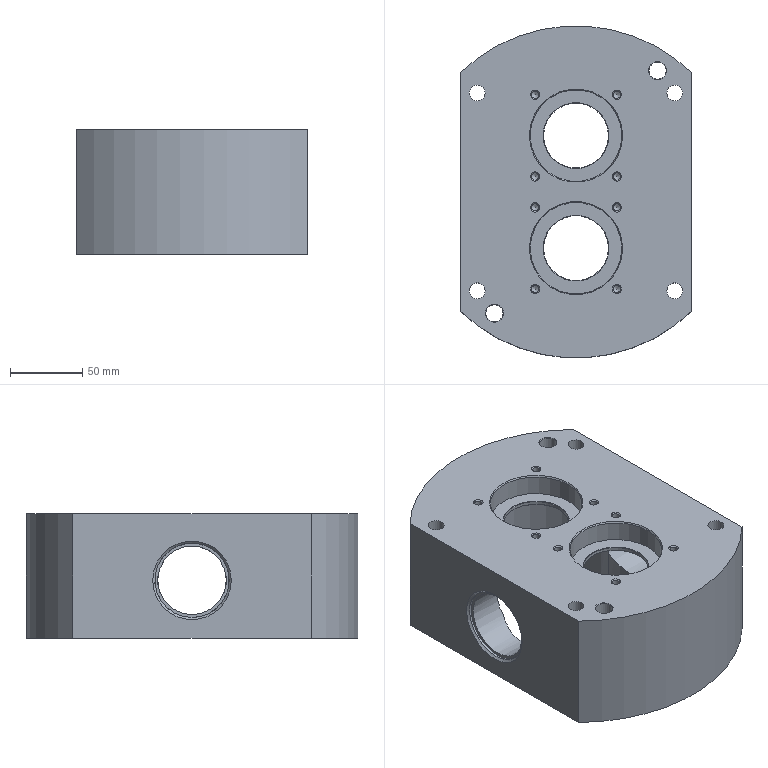NC program | NX | posted with a generic post | part box 160 x 230 x 86 mm
Lines 549 to 1411 of 21365:
(FLOOR_WALL_1 , TOOL : D25R0.5)
N1078 T05 M6
N1080 G54
N1082 G17 G0 G90 X37.526 Y-7.406 B0. C0. S2000 M3
N1084 G43 Z30. H5
N1086 Z1.5
N1088 G94 G1 X37.675 Y-7.443 Z1.496 F1000.
N1090 X38.677 Y-7.553 Z1.47
N1092 X39.685 Y-7.529 Z1.443
N1094 X40.681 Y-7.371 Z1.417
N1096 X41.646 Y-7.082 Z1.39
N1098 X42.565 Y-6.667 Z1.364
N1100 X43.42 Y-6.133 Z1.338
N1102 X44.197 Y-5.49 Z1.311
N1104 X44.881 Y-4.75 Z1.285
N1106 X45.461 Y-3.925 Z1.258
N1108 X45.926 Y-3.031 Z1.232
N1110 X46.063 Y-2.667 Z1.222
N1112 X46.201 Y-2.303 Z1.212
N1114 X46.443 Y-1.325 Z1.185
N1116 X46.553 Y-0.323 Z1.159
N1118 X46.529 Y0.685 Z1.132
N1120 X46.371 Y1.681 Z1.106
N1122 X46.082 Y2.646 Z1.08
N1124 X45.667 Y3.565 Z1.053
N1126 X45.133 Y4.42 Z1.027
N1128 X44.49 Y5.197 Z1.
N1130 X43.75 Y5.881 Z0.974
N1132 X42.925 Y6.461 Z0.948
N1134 X42.031 Y6.926 Z0.921
N1136 X41.667 Y7.063 Z0.911
N1138 X41.303 Y7.201 Z0.901
N1140 X40.396 Y7.43 Z0.876
N1142 X39.468 Y7.546 Z0.852
N1144 X38.532 Z0.827
N1146 X37.604 Y7.43 Z0.803
N1148 X36.697 Y7.201 Z0.778
N1150 X31.081 Y5.08 Z0.621
N1152 X28.829 Y4.375 Z0.559
N1154 X26.534 Y3.823 Z0.498
N1156 X24.207 Y3.427 Z0.436
N1158 X21.859 Y3.189 Z0.374
N1160 X19.5 Y3.109 Z0.312
N1162 X17.141 Y3.189 Z0.25
N1164 X14.793 Y3.427 Z0.189
N1166 X12.466 Y3.823 Z0.127
N1168 X10.171 Y4.375 Z0.065
N1170 X7.919 Y5.08 Z0.003
N1172 X2.303 Y7.201 Z-0.154
N1174 X1.396 Y7.43 Z-0.179
N1176 X0.468 Y7.545 Z-0.203
N1178 X-0.468 Y7.546 Z-0.228
N1180 X-1.396 Y7.43 Z-0.252
N1182 X-2.303 Y7.201 Z-0.277
N1184 X-2.667 Y7.063 Z-0.287
N1186 X-4.901 Y6.22 Z-0.349
N1188 X-7.136 Y5.376 F2200.
N1190 G2 X-31.864 Y5.376 R35.
N1192 G1 X-36.333 Y7.063
N1194 G3 X-36.333 Y-7.063 R-7.55
N1196 G1 X-31.864 Y-5.376
N1198 G2 X-7.136 Y-5.376 R35.
N1200 G1 X-2.667 Y-7.063
N1202 G3 X2.667 Y-7.063 R7.55
N1204 G1 X7.136 Y-5.376
N1206 G2 X31.864 Y-5.376 R35.
N1208 G1 X36.333 Y-7.063
N1210 G3 X36.333 Y7.063 R-7.55
N1212 G1 X31.864 Y5.376
N1214 G2 X7.136 Y5.376 R35.
N1216 G1 X2.667 Y7.063
N1218 G3 X-2.667 Y7.063 R7.55
N1220 G1 X-4.901 Y6.22
N1222 X-11.083 Y22.591
N1224 X-13.318 Y21.747
N1226 G2 X-25.682 Y21.747 R17.5
N1228 G1 X-30.151 Y23.435
N1230 G3 X-30.151 Y-23.435 R-25.05
N1232 G1 X-25.682 Y-21.747
N1234 G2 X-13.318 Y-21.747 R17.5
N1236 G1 X-8.849 Y-23.435
N1238 G3 X8.849 Y-23.435 R25.05
N1240 G1 X13.318 Y-21.747
N1242 G2 X25.682 Y-21.747 R17.5
N1244 G1 X30.151 Y-23.435
N1246 G3 X30.151 Y23.435 R-25.05
N1248 G1 X25.682 Y21.747
N1250 G2 X13.318 Y21.747 R17.5
N1252 G1 X8.849 Y23.435
N1254 G3 X-8.848 Y23.435 R25.05
N1256 G1 X-11.083 Y22.591
N1258 X-17.265 Y38.963
N1260 X-19.5 Y38.119
N1262 X-23.969 Y39.807
N1264 G3 X-23.969 Y-39.807 R-42.55
N1266 G1 X-19.5 Y-38.119
N1268 X-15.031 Y-39.807
N1270 G3 X15.031 Y-39.807 R42.55
N1272 G1 X19.5 Y-38.119
N1274 X23.969 Y-39.807
N1276 G3 X23.969 Y39.807 R-42.55
N1278 G1 X19.5 Y38.119
N1280 X15.031 Y39.807
N1282 G3 X-15.031 Y39.807 R42.55
N1284 G1 X-17.265 Y38.963
N1286 Z1.151
N1288 G0 X37.526 Y-7.406
N1290 G1 X37.675 Y-7.443 Z1.147 F1000.
N1292 X38.677 Y-7.553 Z1.12
N1294 X39.685 Y-7.529 Z1.094
N1296 X40.681 Y-7.371 Z1.068
N1298 X41.646 Y-7.082 Z1.041
N1300 X42.565 Y-6.667 Z1.015
N1302 X43.42 Y-6.133 Z0.988
N1304 X44.197 Y-5.49 Z0.962
N1306 X44.881 Y-4.75 Z0.936
N1308 X45.461 Y-3.925 Z0.909
N1310 X45.926 Y-3.031 Z0.883
N1312 X46.063 Y-2.667 Z0.873
N1314 X46.201 Y-2.303 Z0.862
N1316 X46.443 Y-1.325 Z0.836
N1318 X46.553 Y-0.323 Z0.81
N1320 X46.529 Y0.685 Z0.783
N1322 X46.371 Y1.681 Z0.757
N1324 X46.082 Y2.646 Z0.73
N1326 X45.667 Y3.565 Z0.704
N1328 X45.133 Y4.42 Z0.678
N1330 X44.49 Y5.197 Z0.651
N1332 X43.75 Y5.881 Z0.625
N1334 X42.925 Y6.461 Z0.598
N1336 X42.031 Y6.926 Z0.572
N1338 X41.667 Y7.063 Z0.562
N1340 X41.303 Y7.201 Z0.552
N1342 X40.396 Y7.43 Z0.527
N1344 X39.468 Y7.546 Z0.503
N1346 X38.532 Z0.478
N1348 X37.604 Y7.43 Z0.454
N1350 X36.697 Y7.201 Z0.429
N1352 X31.081 Y5.08 Z0.272
N1354 X28.829 Y4.375 Z0.21
N1356 X26.534 Y3.823 Z0.148
N1358 X24.207 Y3.427 Z0.087
N1360 X21.859 Y3.189 Z0.025
N1362 X19.5 Y3.109 Z-0.037
N1364 X17.141 Y3.189 Z-0.099
N1366 X14.793 Y3.427 Z-0.161
N1368 X12.466 Y3.823 Z-0.222
N1370 X10.171 Y4.375 Z-0.284
N1372 X7.919 Y5.08 Z-0.346
N1374 X2.303 Y7.201 Z-0.503
N1376 X1.396 Y7.43 Z-0.528
N1378 X0.468 Y7.545 Z-0.552
N1380 X-0.468 Y7.546 Z-0.577
N1382 X-1.396 Y7.43 Z-0.601
N1384 X-2.303 Y7.201 Z-0.626
N1386 X-2.667 Y7.063 Z-0.636
N1388 X-4.901 Y6.22 Z-0.698
N1390 X-7.136 Y5.376 F2200.
N1392 G2 X-31.864 Y5.376 R35.
N1394 G1 X-36.333 Y7.063
N1396 G3 X-36.333 Y-7.063 R-7.55
N1398 G1 X-31.864 Y-5.376
N1400 G2 X-7.136 Y-5.376 R35.
N1402 G1 X-2.667 Y-7.063
N1404 G3 X2.667 Y-7.063 R7.55
N1406 G1 X7.136 Y-5.376
N1408 G2 X31.864 Y-5.376 R35.
N1410 G1 X36.333 Y-7.063
N1412 G3 X36.333 Y7.063 R-7.55
N1414 G1 X31.864 Y5.376
N1416 G2 X7.136 Y5.376 R35.
N1418 G1 X2.667 Y7.063
N1420 G3 X-2.667 Y7.063 R7.55
N1422 G1 X-4.901 Y6.22
N1424 X-11.083 Y22.591
N1426 X-13.318 Y21.747
N1428 G2 X-25.682 Y21.747 R17.5
N1430 G1 X-30.151 Y23.435
N1432 G3 X-30.151 Y-23.435 R-25.05
N1434 G1 X-25.682 Y-21.747
N1436 G2 X-13.318 Y-21.747 R17.5
N1438 G1 X-8.849 Y-23.435
N1440 G3 X8.849 Y-23.435 R25.05
N1442 G1 X13.318 Y-21.747
N1444 G2 X25.682 Y-21.747 R17.5
N1446 G1 X30.151 Y-23.435
N1448 G3 X30.151 Y23.435 R-25.05
N1450 G1 X25.682 Y21.747
N1452 G2 X13.318 Y21.747 R17.5
N1454 G1 X8.849 Y23.435
N1456 G3 X-8.848 Y23.435 R25.05
N1458 G1 X-11.083 Y22.591
N1460 X-17.265 Y38.963
N1462 X-19.5 Y38.119
N1464 X-23.969 Y39.807
N1466 G3 X-23.969 Y-39.807 R-42.55
N1468 G1 X-19.5 Y-38.119
N1470 X-15.031 Y-39.807
N1472 G3 X15.031 Y-39.807 R42.55
N1474 G1 X19.5 Y-38.119
N1476 X23.969 Y-39.807
N1478 G3 X23.969 Y39.807 R-42.55
N1480 G1 X19.5 Y38.119
N1482 X15.031 Y39.807
N1484 G3 X-15.031 Y39.807 R42.55
N1486 G1 X-17.265 Y38.963
N1488 Z0.802
N1490 G0 X37.526 Y-7.406
N1492 G1 X37.675 Y-7.443 Z0.798 F1000.
N1494 X38.677 Y-7.553 Z0.771
N1496 X39.685 Y-7.529 Z0.745
N1498 X40.681 Y-7.371 Z0.718
N1500 X41.646 Y-7.082 Z0.692
N1502 X42.565 Y-6.667 Z0.666
N1504 X43.42 Y-6.133 Z0.639
N1506 X44.197 Y-5.49 Z0.613
N1508 X44.881 Y-4.75 Z0.586
N1510 X45.461 Y-3.925 Z0.56
N1512 X45.926 Y-3.031 Z0.534
N1514 X46.063 Y-2.667 Z0.523
N1516 X46.201 Y-2.303 Z0.513
N1518 X46.443 Y-1.325 Z0.487
N1520 X46.553 Y-0.323 Z0.46
N1522 X46.529 Y0.685 Z0.434
N1524 X46.371 Y1.681 Z0.408
N1526 X46.082 Y2.646 Z0.381
N1528 X45.667 Y3.565 Z0.355
N1530 X45.133 Y4.42 Z0.328
N1532 X44.49 Y5.197 Z0.302
N1534 X43.75 Y5.881 Z0.276
N1536 X42.925 Y6.461 Z0.249
N1538 X42.031 Y6.926 Z0.223
N1540 X41.667 Y7.063 Z0.213
N1542 X41.303 Y7.201 Z0.202
N1544 X40.396 Y7.43 Z0.178
N1546 X39.468 Y7.546 Z0.153
N1548 X38.532 Z0.129
N1550 X37.604 Y7.43 Z0.104
N1552 X36.697 Y7.201 Z0.08
N1554 X31.081 Y5.08 Z-0.077
N1556 X28.829 Y4.375 Z-0.139
N1558 X26.534 Y3.823 Z-0.201
N1560 X24.207 Y3.427 Z-0.263
N1562 X21.859 Y3.189 Z-0.324
N1564 X19.5 Y3.109 Z-0.386
N1566 X17.141 Y3.189 Z-0.448
N1568 X14.793 Y3.427 Z-0.51
N1570 X12.466 Y3.823 Z-0.572
N1572 X10.171 Y4.375 Z-0.633
N1574 X7.919 Y5.08 Z-0.695
N1576 X2.303 Y7.201 Z-0.852
N1578 X1.396 Y7.43 Z-0.877
N1580 X0.468 Y7.545 Z-0.901
N1582 X-0.468 Y7.546 Z-0.926
N1584 X-1.396 Y7.43 Z-0.95
N1586 X-2.303 Y7.201 Z-0.975
N1588 X-2.667 Y7.063 Z-0.985
N1590 X-4.901 Y6.22 Z-1.048
N1592 X-7.136 Y5.376 F2200.
N1594 G2 X-31.864 Y5.376 R35.
N1596 G1 X-36.333 Y7.063
N1598 G3 X-36.333 Y-7.063 R-7.55
N1600 G1 X-31.864 Y-5.376
N1602 G2 X-7.136 Y-5.376 R35.
N1604 G1 X-2.667 Y-7.063
N1606 G3 X2.667 Y-7.063 R7.55
N1608 G1 X7.136 Y-5.376
N1610 G2 X31.864 Y-5.376 R35.
N1612 G1 X36.333 Y-7.063
N1614 G3 X36.333 Y7.063 R-7.55
N1616 G1 X31.864 Y5.376
N1618 G2 X7.136 Y5.376 R35.
N1620 G1 X2.667 Y7.063
N1622 G3 X-2.667 Y7.063 R7.55
N1624 G1 X-4.901 Y6.22
N1626 X-11.083 Y22.591
N1628 X-13.318 Y21.747
N1630 G2 X-25.682 Y21.747 R17.5
N1632 G1 X-30.151 Y23.435
N1634 G3 X-30.151 Y-23.435 R-25.05
N1636 G1 X-25.682 Y-21.747
N1638 G2 X-13.318 Y-21.747 R17.5
N1640 G1 X-8.849 Y-23.435
N1642 G3 X8.849 Y-23.435 R25.05
N1644 G1 X13.318 Y-21.747
N1646 G2 X25.682 Y-21.747 R17.5
N1648 G1 X30.151 Y-23.435
N1650 G3 X30.151 Y23.435 R-25.05
N1652 G1 X25.682 Y21.747
N1654 G2 X13.318 Y21.747 R17.5
N1656 G1 X8.849 Y23.435
N1658 G3 X-8.848 Y23.435 R25.05
N1660 G1 X-11.083 Y22.591
N1662 X-17.265 Y38.963
N1664 X-19.5 Y38.119
N1666 X-23.969 Y39.807
N1668 G3 X-23.969 Y-39.807 R-42.55
N1670 G1 X-19.5 Y-38.119
N1672 X-15.031 Y-39.807
N1674 G3 X15.031 Y-39.807 R42.55
N1676 G1 X19.5 Y-38.119
N1678 X23.969 Y-39.807
N1680 G3 X23.969 Y39.807 R-42.55
N1682 G1 X19.5 Y38.119
N1684 X15.031 Y39.807
N1686 G3 X-15.031 Y39.807 R42.55
N1688 G1 X-17.265 Y38.963
N1690 Z0.452
N1692 G0 X37.526 Y-7.406
N1694 G1 X37.675 Y-7.443 Z0.448 F1000.
N1696 X38.677 Y-7.553 Z0.422
N1698 X39.685 Y-7.529 Z0.396
N1700 X40.681 Y-7.371 Z0.369
N1702 X41.646 Y-7.082 Z0.343
N1704 X42.565 Y-6.667 Z0.316
N1706 X43.42 Y-6.133 Z0.29
N1708 X44.197 Y-5.49 Z0.264
N1710 X44.881 Y-4.75 Z0.237
N1712 X45.461 Y-3.925 Z0.211
N1714 X45.926 Y-3.031 Z0.184
N1716 X46.063 Y-2.667 Z0.174
N1718 X46.201 Y-2.303 Z0.164
N1720 X46.443 Y-1.325 Z0.138
N1722 X46.553 Y-0.323 Z0.111
N1724 X46.529 Y0.685 Z0.085
N1726 X46.371 Y1.681 Z0.058
N1728 X46.082 Y2.646 Z0.032
N1730 X45.667 Y3.565 Z0.006
N1732 X45.133 Y4.42 Z-0.021
N1734 X44.49 Y5.197 Z-0.047
N1736 X43.75 Y5.881 Z-0.074
N1738 X42.925 Y6.461 Z-0.1
N1740 X42.031 Y6.926 Z-0.126
N1742 X41.667 Y7.063 Z-0.137
N1744 X41.303 Y7.201 Z-0.147
N1746 X40.396 Y7.43 Z-0.171
N1748 X39.468 Y7.546 Z-0.196
N1750 X38.532 Z-0.22
N1752 X37.604 Y7.43 Z-0.245
N1754 X36.697 Y7.201 Z-0.269
N1756 X31.081 Y5.08 Z-0.426
N1758 X28.829 Y4.375 Z-0.488
N1760 X26.534 Y3.823 Z-0.55
N1762 X24.207 Y3.427 Z-0.612
N1764 X21.859 Y3.189 Z-0.674
N1766 X19.5 Y3.109 Z-0.735
N1768 X17.141 Y3.189 Z-0.797
N1770 X14.793 Y3.427 Z-0.859
N1772 X12.466 Y3.823 Z-0.921
N1774 X10.171 Y4.375 Z-0.983
N1776 X7.919 Y5.08 Z-1.045
N1778 X2.303 Y7.201 Z-1.202
N1780 X1.396 Y7.43 Z-1.226
N1782 X0.468 Y7.545 Z-1.251
N1784 X-0.468 Y7.546 Z-1.275
N1786 X-1.396 Y7.43 Z-1.3
N1788 X-2.303 Y7.201 Z-1.324
N1790 X-2.667 Y7.063 Z-1.334
N1792 X-4.901 Y6.22 Z-1.397
N1794 X-7.136 Y5.376 F2200.
N1796 G2 X-31.864 Y5.376 R35.
N1798 G1 X-36.333 Y7.063
N1800 G3 X-36.333 Y-7.063 R-7.55
N1802 G1 X-31.864 Y-5.376
N1804 G2 X-7.136 Y-5.376 R35.
N1806 G1 X-2.667 Y-7.063
N1808 G3 X2.667 Y-7.063 R7.55
N1810 G1 X7.136 Y-5.376
N1812 G2 X31.864 Y-5.376 R35.
N1814 G1 X36.333 Y-7.063
N1816 G3 X36.333 Y7.063 R-7.55
N1818 G1 X31.864 Y5.376
N1820 G2 X7.136 Y5.376 R35.
N1822 G1 X2.667 Y7.063
N1824 G3 X-2.667 Y7.063 R7.55
N1826 G1 X-4.901 Y6.22
N1828 X-11.083 Y22.591
N1830 X-13.318 Y21.747
N1832 G2 X-25.682 Y21.747 R17.5
N1834 G1 X-30.151 Y23.435
N1836 G3 X-30.151 Y-23.435 R-25.05
N1838 G1 X-25.682 Y-21.747
N1840 G2 X-13.318 Y-21.747 R17.5
N1842 G1 X-8.849 Y-23.435
N1844 G3 X8.849 Y-23.435 R25.05
N1846 G1 X13.318 Y-21.747
N1848 G2 X25.682 Y-21.747 R17.5
N1850 G1 X30.151 Y-23.435
N1852 G3 X30.151 Y23.435 R-25.05
N1854 G1 X25.682 Y21.747
N1856 G2 X13.318 Y21.747 R17.5
N1858 G1 X8.849 Y23.435
N1860 G3 X-8.848 Y23.435 R25.05
N1862 G1 X-11.083 Y22.591
N1864 X-17.265 Y38.963
N1866 X-19.5 Y38.119
N1868 X-23.969 Y39.807
N1870 G3 X-23.969 Y-39.807 R-42.55
N1872 G1 X-19.5 Y-38.119
N1874 X-15.031 Y-39.807
N1876 G3 X15.031 Y-39.807 R42.55
N1878 G1 X19.5 Y-38.119
N1880 X23.969 Y-39.807
N1882 G3 X23.969 Y39.807 R-42.55
N1884 G1 X19.5 Y38.119
N1886 X15.031 Y39.807
N1888 G3 X-15.031 Y39.807 R42.55
N1890 G1 X-17.265 Y38.963
N1892 Z0.103
N1894 G0 X37.526 Y-7.406
N1896 G1 X37.675 Y-7.443 Z0.099 F1000.
N1898 X38.677 Y-7.553 Z0.073
N1900 X39.685 Y-7.529 Z0.046
N1902 X40.681 Y-7.371 Z0.02
N1904 X41.646 Y-7.082 Z-0.007
N1906 X42.565 Y-6.667 Z-0.033
N1908 X43.42 Y-6.133 Z-0.059
N1910 X44.197 Y-5.49 Z-0.086
N1912 X44.881 Y-4.75 Z-0.112
N1914 X45.461 Y-3.925 Z-0.139
N1916 X45.926 Y-3.031 Z-0.165
N1918 X46.063 Y-2.667 Z-0.175
N1920 X46.201 Y-2.303 Z-0.185
N1922 X46.443 Y-1.325 Z-0.212
N1924 X46.553 Y-0.323 Z-0.238
N1926 X46.529 Y0.685 Z-0.264
N1928 X46.371 Y1.681 Z-0.291
N1930 X46.082 Y2.646 Z-0.317
N1932 X45.667 Y3.565 Z-0.344
N1934 X45.133 Y4.42 Z-0.37
N1936 X44.49 Y5.197 Z-0.396
N1938 X43.75 Y5.881 Z-0.423
N1940 X42.925 Y6.461 Z-0.449
N1942 X42.031 Y6.926 Z-0.476
N1944 X41.667 Y7.063 Z-0.486
N1946 X41.303 Y7.201 Z-0.496
N1948 X40.396 Y7.43 Z-0.521
N1950 X39.468 Y7.546 Z-0.545
N1952 X38.532 Z-0.57
N1954 X37.604 Y7.43 Z-0.594
N1956 X36.697 Y7.201 Z-0.619
N1958 X31.081 Y5.08 Z-0.776
N1960 X28.829 Y4.375 Z-0.838
N1962 X26.534 Y3.823 Z-0.899
N1964 X24.207 Y3.427 Z-0.961
N1966 X21.859 Y3.189 Z-1.023
N1968 X19.5 Y3.109 Z-1.085
N1970 X17.141 Y3.189 Z-1.147
N1972 X14.793 Y3.427 Z-1.208
N1974 X12.466 Y3.823 Z-1.27
N1976 X10.171 Y4.375 Z-1.332
N1978 X7.919 Y5.08 Z-1.394
N1980 X2.303 Y7.201 Z-1.551
N1982 X1.396 Y7.43 Z-1.575
N1984 X0.468 Y7.545 Z-1.6
N1986 X-0.468 Y7.546 Z-1.624
N1988 X-1.396 Y7.43 Z-1.649
N1990 X-2.303 Y7.201 Z-1.673
N1992 X-2.667 Y7.063 Z-1.684
N1994 X-4.901 Y6.22 Z-1.746
N1996 X-7.136 Y5.376 F2200.
N1998 G2 X-31.864 Y5.376 R35.
N2000 G1 X-36.333 Y7.063
N2002 G3 X-36.333 Y-7.063 R-7.55
N2004 G1 X-31.864 Y-5.376
N2006 G2 X-7.136 Y-5.376 R35.
N2008 G1 X-2.667 Y-7.063
N2010 G3 X2.667 Y-7.063 R7.55
N2012 G1 X7.136 Y-5.376
N2014 G2 X31.864 Y-5.376 R35.
N2016 G1 X36.333 Y-7.063
N2018 G3 X36.333 Y7.063 R-7.55
N2020 G1 X31.864 Y5.376
N2022 G2 X7.136 Y5.376 R35.
N2024 G1 X2.667 Y7.063
N2026 G3 X-2.667 Y7.063 R7.55
N2028 G1 X-4.901 Y6.22
N2030 X-11.083 Y22.591
N2032 X-13.318 Y21.747
N2034 G2 X-25.682 Y21.747 R17.5
N2036 G1 X-30.151 Y23.435
N2038 G3 X-30.151 Y-23.435 R-25.05
N2040 G1 X-25.682 Y-21.747
N2042 G2 X-13.318 Y-21.747 R17.5
N2044 G1 X-8.849 Y-23.435
N2046 G3 X8.849 Y-23.435 R25.05
N2048 G1 X13.318 Y-21.747
N2050 G2 X25.682 Y-21.747 R17.5
N2052 G1 X30.151 Y-23.435
N2054 G3 X30.151 Y23.435 R-25.05
N2056 G1 X25.682 Y21.747
N2058 G2 X13.318 Y21.747 R17.5
N2060 G1 X8.849 Y23.435
N2062 G3 X-8.848 Y23.435 R25.05
N2064 G1 X-11.083 Y22.591
N2066 X-17.265 Y38.963
N2068 X-19.5 Y38.119
N2070 X-23.969 Y39.807
N2072 G3 X-23.969 Y-39.807 R-42.55
N2074 G1 X-19.5 Y-38.119
N2076 X-15.031 Y-39.807
N2078 G3 X15.031 Y-39.807 R42.55
N2080 G1 X19.5 Y-38.119
N2082 X23.969 Y-39.807
N2084 G3 X23.969 Y39.807 R-42.55
N2086 G1 X19.5 Y38.119
N2088 X15.031 Y39.807
N2090 G3 X-15.031 Y39.807 R42.55
N2092 G1 X-17.265 Y38.963
N2094 Z-0.246
N2096 G0 X37.526 Y-7.406
N2098 G1 X37.675 Y-7.443 Z-0.25 F1000.
N2100 X38.677 Y-7.553 Z-0.277
N2102 X39.685 Y-7.529 Z-0.303
N2104 X40.681 Y-7.371 Z-0.329
N2106 X41.646 Y-7.082 Z-0.356
N2108 X42.565 Y-6.667 Z-0.382
N2110 X43.42 Y-6.133 Z-0.409
N2112 X44.197 Y-5.49 Z-0.435
N2114 X44.881 Y-4.75 Z-0.461
N2116 X45.461 Y-3.925 Z-0.488
N2118 X45.926 Y-3.031 Z-0.514
N2120 X46.063 Y-2.667 Z-0.524
N2122 X46.201 Y-2.303 Z-0.535
N2124 X46.443 Y-1.325 Z-0.561
N2126 X46.553 Y-0.323 Z-0.587
N2128 X46.529 Y0.685 Z-0.614
N2130 X46.371 Y1.681 Z-0.64
N2132 X46.082 Y2.646 Z-0.666
N2134 X45.667 Y3.565 Z-0.693
N2136 X45.133 Y4.42 Z-0.719
N2138 X44.49 Y5.197 Z-0.746
N2140 X43.75 Y5.881 Z-0.772
N2142 X42.925 Y6.461 Z-0.798
N2144 X42.031 Y6.926 Z-0.825
N2146 X41.667 Y7.063 Z-0.835
N2148 X41.303 Y7.201 Z-0.845
N2150 X40.396 Y7.43 Z-0.87
N2152 X39.468 Y7.546 Z-0.894
N2154 X38.532 Z-0.919
N2156 X37.604 Y7.43 Z-0.943
N2158 X36.697 Y7.201 Z-0.968
N2160 X31.081 Y5.08 Z-1.125
N2162 X28.829 Y4.375 Z-1.187
N2164 X26.534 Y3.823 Z-1.249
N2166 X24.207 Y3.427 Z-1.31
N2168 X21.859 Y3.189 Z-1.372
N2170 X19.5 Y3.109 Z-1.434
N2172 X17.141 Y3.189 Z-1.496
N2174 X14.793 Y3.427 Z-1.558
N2176 X12.466 Y3.823 Z-1.619
N2178 X10.171 Y4.375 Z-1.681
N2180 X7.919 Y5.08 Z-1.743
N2182 X2.303 Y7.201 Z-1.9
N2184 X1.396 Y7.43 Z-1.925
N2186 X0.468 Y7.545 Z-1.949
N2188 X-0.468 Y7.546 Z-1.974
N2190 X-1.396 Y7.43 Z-1.998
N2192 X-2.303 Y7.201 Z-2.023
N2194 X-2.667 Y7.063 Z-2.033
N2196 X-4.901 Y6.22 Z-2.095
N2198 X-7.136 Y5.376 F2200.
N2200 G2 X-31.864 Y5.376 R35.
N2202 G1 X-36.333 Y7.063
N2204 G3 X-36.333 Y-7.063 R-7.55
N2206 G1 X-31.864 Y-5.376
N2208 G2 X-7.136 Y-5.376 R35.
N2210 G1 X-2.667 Y-7.063
N2212 G3 X2.667 Y-7.063 R7.55
N2214 G1 X7.136 Y-5.376
N2216 G2 X31.864 Y-5.376 R35.
N2218 G1 X36.333 Y-7.063
N2220 G3 X36.333 Y7.063 R-7.55
N2222 G1 X31.864 Y5.376
N2224 G2 X7.136 Y5.376 R35.
N2226 G1 X2.667 Y7.063
N2228 G3 X-2.667 Y7.063 R7.55
N2230 G1 X-4.901 Y6.22
N2232 X-11.083 Y22.591
N2234 X-13.318 Y21.747
N2236 G2 X-25.682 Y21.747 R17.5
N2238 G1 X-30.151 Y23.435
N2240 G3 X-30.151 Y-23.435 R-25.05
N2242 G1 X-25.682 Y-21.747
N2244 G2 X-13.318 Y-21.747 R17.5
N2246 G1 X-8.849 Y-23.435
N2248 G3 X8.849 Y-23.435 R25.05
N2250 G1 X13.318 Y-21.747
N2252 G2 X25.682 Y-21.747 R17.5
N2254 G1 X30.151 Y-23.435
N2256 G3 X30.151 Y23.435 R-25.05
N2258 G1 X25.682 Y21.747
N2260 G2 X13.318 Y21.747 R17.5
N2262 G1 X8.849 Y23.435
N2264 G3 X-8.848 Y23.435 R25.05
N2266 G1 X-11.083 Y22.591
N2268 X-17.265 Y38.963
N2270 X-19.5 Y38.119
N2272 X-23.969 Y39.807
N2274 G3 X-23.969 Y-39.807 R-42.55
N2276 G1 X-19.5 Y-38.119
N2278 X-15.031 Y-39.807
N2280 G3 X15.031 Y-39.807 R42.55
N2282 G1 X19.5 Y-38.119
N2284 X23.969 Y-39.807
N2286 G3 X23.969 Y39.807 R-42.55
N2288 G1 X19.5 Y38.119
N2290 X15.031 Y39.807
N2292 G3 X-15.031 Y39.807 R42.55
N2294 G1 X-17.265 Y38.963
N2296 Z-0.595
N2298 G0 X37.526 Y-7.406
N2300 G1 X37.675 Y-7.443 Z-0.599 F1000.
N2302 X38.677 Y-7.553 Z-0.626
N2304 X39.685 Y-7.529 Z-0.652
N2306 X40.681 Y-7.371 Z-0.679
N2308 X41.646 Y-7.082 Z-0.705
N2310 X42.565 Y-6.667 Z-0.731
N2312 X43.42 Y-6.133 Z-0.758
N2314 X44.197 Y-5.49 Z-0.784
N2316 X44.881 Y-4.75 Z-0.811
N2318 X45.461 Y-3.925 Z-0.837
N2320 X45.926 Y-3.031 Z-0.863
N2322 X46.063 Y-2.667 Z-0.874
N2324 X46.201 Y-2.303 Z-0.884
N2326 X46.443 Y-1.325 Z-0.91
N2328 X46.553 Y-0.323 Z-0.937
N2330 X46.529 Y0.685 Z-0.963
N2332 X46.371 Y1.681 Z-0.989
N2334 X46.082 Y2.646 Z-1.016
N2336 X45.667 Y3.565 Z-1.042
N2338 X45.133 Y4.42 Z-1.069
N2340 X44.49 Y5.197 Z-1.095
N2342 X43.75 Y5.881 Z-1.121
N2344 X42.925 Y6.461 Z-1.148
N2346 X42.031 Y6.926 Z-1.174
N2348 X41.667 Y7.063 Z-1.184
N2350 X41.303 Y7.201 Z-1.194
N2352 X40.396 Y7.43 Z-1.219
N2354 X39.468 Y7.546 Z-1.243
N2356 X38.532 Z-1.268
N2358 X37.604 Y7.43 Z-1.292
N2360 X36.697 Y7.201 Z-1.317
N2362 X31.081 Y5.08 Z-1.474
N2364 X28.829 Y4.375 Z-1.536
N2366 X26.534 Y3.823 Z-1.598
N2368 X24.207 Y3.427 Z-1.66
N2370 X21.859 Y3.189 Z-1.721
N2372 X19.5 Y3.109 Z-1.783
N2374 X17.141 Y3.189 Z-1.845
N2376 X14.793 Y3.427 Z-1.907
N2378 X12.466 Y3.823 Z-1.969
N2380 X10.171 Y4.375 Z-2.03
N2382 X7.919 Y5.08 Z-2.092
N2384 X2.303 Y7.201 Z-2.249
N2386 X1.396 Y7.43 Z-2.274
N2388 X0.468 Y7.545 Z-2.298
N2390 X-0.468 Y7.546 Z-2.323
N2392 X-1.396 Y7.43 Z-2.347
N2394 X-2.303 Y7.201 Z-2.372
N2396 X-2.667 Y7.063 Z-2.382
N2398 X-4.901 Y6.22 Z-2.445
N2400 X-7.136 Y5.376 F2200.
N2402 G2 X-31.864 Y5.376 R35.
N2404 G1 X-36.333 Y7.063
N2406 G3 X-36.333 Y-7.063 R-7.55
N2408 G1 X-31.864 Y-5.376
N2410 G2 X-7.136 Y-5.376 R35.
N2412 G1 X-2.667 Y-7.063
N2414 G3 X2.667 Y-7.063 R7.55
N2416 G1 X7.136 Y-5.376
N2418 G2 X31.864 Y-5.376 R35.
N2420 G1 X36.333 Y-7.063
N2422 G3 X36.333 Y7.063 R-7.55
N2424 G1 X31.864 Y5.376
N2426 G2 X7.136 Y5.376 R35.
N2428 G1 X2.667 Y7.063
N2430 G3 X-2.667 Y7.063 R7.55
N2432 G1 X-4.901 Y6.22
N2434 X-11.083 Y22.591
N2436 X-13.318 Y21.747
N2438 G2 X-25.682 Y21.747 R17.5
N2440 G1 X-30.151 Y23.435
N2442 G3 X-30.151 Y-23.435 R-25.05
N2444 G1 X-25.682 Y-21.747
N2446 G2 X-13.318 Y-21.747 R17.5
N2448 G1 X-8.849 Y-23.435
N2450 G3 X8.849 Y-23.435 R25.05
N2452 G1 X13.318 Y-21.747
N2454 G2 X25.682 Y-21.747 R17.5
N2456 G1 X30.151 Y-23.435
N2458 G3 X30.151 Y23.435 R-25.05
N2460 G1 X25.682 Y21.747
N2462 G2 X13.318 Y21.747 R17.5
N2464 G1 X8.849 Y23.435
N2466 G3 X-8.848 Y23.435 R25.05
N2468 G1 X-11.083 Y22.591
N2470 X-17.265 Y38.963
N2472 X-19.5 Y38.119
N2474 X-23.969 Y39.807
N2476 G3 X-23.969 Y-39.807 R-42.55
N2478 G1 X-19.5 Y-38.119
N2480 X-15.031 Y-39.807
N2482 G3 X15.031 Y-39.807 R42.55
N2484 G1 X19.5 Y-38.119
N2486 X23.969 Y-39.807
N2488 G3 X23.969 Y39.807 R-42.55
N2490 G1 X19.5 Y38.119
N2492 X15.031 Y39.807
N2494 G3 X-15.031 Y39.807 R42.55
N2496 G1 X-17.265 Y38.963
N2498 Z-0.945
N2500 G0 X37.526 Y-7.406
N2502 G1 X37.675 Y-7.443 Z-0.949 F1000.
N2504 X38.677 Y-7.553 Z-0.975
N2506 X39.685 Y-7.529 Z-1.001
N2508 X40.681 Y-7.371 Z-1.028
N2510 X41.646 Y-7.082 Z-1.054
N2512 X42.565 Y-6.667 Z-1.081
N2514 X43.42 Y-6.133 Z-1.107
N2516 X44.197 Y-5.49 Z-1.133
N2518 X44.881 Y-4.75 Z-1.16
N2520 X45.461 Y-3.925 Z-1.186
N2522 X45.926 Y-3.031 Z-1.213
N2524 X46.063 Y-2.667 Z-1.223
N2526 X46.201 Y-2.303 Z-1.233
N2528 X46.443 Y-1.325 Z-1.259
N2530 X46.553 Y-0.323 Z-1.286
N2532 X46.529 Y0.685 Z-1.312
N2534 X46.371 Y1.681 Z-1.339
N2536 X46.082 Y2.646 Z-1.365
N2538 X45.667 Y3.565 Z-1.391
N2540 X45.133 Y4.42 Z-1.418
N2542 X44.49 Y5.197 Z-1.444
N2544 X43.75 Y5.881 Z-1.471
N2546 X42.925 Y6.461 Z-1.497
N2548 X42.031 Y6.926 Z-1.523
N2550 X41.667 Y7.063 Z-1.534
N2552 X41.303 Y7.201 Z-1.544
N2554 X40.396 Y7.43 Z-1.568
N2556 X39.468 Y7.546 Z-1.593
N2558 X38.532 Z-1.617
N2560 X37.604 Y7.43 Z-1.642
N2562 X36.697 Y7.201 Z-1.666
N2564 X31.081 Y5.08 Z-1.823
N2566 X28.829 Y4.375 Z-1.885
N2568 X26.534 Y3.823 Z-1.947
N2570 X24.207 Y3.427 Z-2.009
N2572 X21.859 Y3.189 Z-2.071
N2574 X19.5 Y3.109 Z-2.132
N2576 X17.141 Y3.189 Z-2.194
N2578 X14.793 Y3.427 Z-2.256
N2580 X12.466 Y3.823 Z-2.318
N2582 X10.171 Y4.375 Z-2.38
N2584 X7.919 Y5.08 Z-2.441
N2586 X2.303 Y7.201 Z-2.599
N2588 X1.396 Y7.43 Z-2.623
N2590 X0.468 Y7.545 Z-2.648
N2592 X-0.468 Y7.546 Z-2.672
N2594 X-1.396 Y7.43 Z-2.697
N2596 X-2.303 Y7.201 Z-2.721
N2598 X-2.667 Y7.063 Z-2.731
N2600 X-4.901 Y6.22 Z-2.794
N2602 X-7.136 Y5.376 F2200.
N2604 G2 X-31.864 Y5.376 R35.
N2606 G1 X-36.333 Y7.063
N2608 G3 X-36.333 Y-7.063 R-7.55
N2610 G1 X-31.864 Y-5.376
N2612 G2 X-7.136 Y-5.376 R35.
N2614 G1 X-2.667 Y-7.063
N2616 G3 X2.667 Y-7.063 R7.55
N2618 G1 X7.136 Y-5.376
N2620 G2 X31.864 Y-5.376 R35.
N2622 G1 X36.333 Y-7.063
N2624 G3 X36.333 Y7.063 R-7.55
N2626 G1 X31.864 Y5.376
N2628 G2 X7.136 Y5.376 R35.
N2630 G1 X2.667 Y7.063
N2632 G3 X-2.667 Y7.063 R7.55
N2634 G1 X-4.901 Y6.22
N2636 X-11.083 Y22.591
N2638 X-13.318 Y21.747
N2640 G2 X-25.682 Y21.747 R17.5
N2642 G1 X-30.151 Y23.435
N2644 G3 X-30.151 Y-23.435 R-25.05
N2646 G1 X-25.682 Y-21.747
N2648 G2 X-13.318 Y-21.747 R17.5
N2650 G1 X-8.849 Y-23.435
N2652 G3 X8.849 Y-23.435 R25.05
N2654 G1 X13.318 Y-21.747
N2656 G2 X25.682 Y-21.747 R17.5
N2658 G1 X30.151 Y-23.435
N2660 G3 X30.151 Y23.435 R-25.05
N2662 G1 X25.682 Y21.747
N2664 G2 X13.318 Y21.747 R17.5
N2666 G1 X8.849 Y23.435
N2668 G3 X-8.848 Y23.435 R25.05
N2670 G1 X-11.083 Y22.591
N2672 X-17.265 Y38.963
N2674 X-19.5 Y38.119
N2676 X-23.969 Y39.807
N2678 G3 X-23.969 Y-39.807 R-42.55
N2680 G1 X-19.5 Y-38.119
N2682 X-15.031 Y-39.807
N2684 G3 X15.031 Y-39.807 R42.55
N2686 G1 X19.5 Y-38.119
N2688 X23.969 Y-39.807
N2690 G3 X23.969 Y39.807 R-42.55
N2692 G1 X19.5 Y38.119
N2694 X15.031 Y39.807
N2696 G3 X-15.031 Y39.807 R42.55
N2698 G1 X-17.265 Y38.963
N2700 Z-1.294
N2702 G0 X37.526 Y-7.406
N2704 G1 X37.675 Y-7.443 Z-1.298 F1000.
N2706 X38.677 Y-7.553 Z-1.324
N2708 X39.685 Y-7.529 Z-1.351
N2710 X40.681 Y-7.371 Z-1.377
N2712 X41.646 Y-7.082 Z-1.403
N2714 X42.565 Y-6.667 Z-1.43
N2716 X43.42 Y-6.133 Z-1.456
N2718 X44.197 Y-5.49 Z-1.483
N2720 X44.881 Y-4.75 Z-1.509
N2722 X45.461 Y-3.925 Z-1.535
N2724 X45.926 Y-3.031 Z-1.562
N2726 X46.063 Y-2.667 Z-1.572
N2728 X46.201 Y-2.303 Z-1.582
N2730 X46.443 Y-1.325 Z-1.609
N2732 X46.553 Y-0.323 Z-1.635
N2734 X46.529 Y0.685 Z-1.661
N2736 X46.371 Y1.681 Z-1.688
N2738 X46.082 Y2.646 Z-1.714
N2740 X45.667 Y3.565 Z-1.741
N2742 X45.133 Y4.42 Z-1.767
N2744 X44.49 Y5.197 Z-1.793
N2746 X43.75 Y5.881 Z-1.82
N2748 X42.925 Y6.461 Z-1.846
N2750 X42.031 Y6.926 Z-1.873
N2752 X41.667 Y7.063 Z-1.883
N2754 X41.303 Y7.201 Z-1.893
N2756 X40.396 Y7.43 Z-1.917
N2758 X39.468 Y7.546 Z-1.942
N2760 X38.532 Z-1.966
N2762 X37.604 Y7.43 Z-1.991
N2764 X36.697 Y7.201 Z-2.015
N2766 X31.081 Y5.08 Z-2.173
N2768 X28.829 Y4.375 Z-2.234
N2770 X26.534 Y3.823 Z-2.296
N2772 X24.207 Y3.427 Z-2.358
N2774 X21.859 Y3.189 Z-2.42
N2776 X19.5 Y3.109 Z-2.482
N2778 X17.141 Y3.189 Z-2.543
N2780 X14.793 Y3.427 Z-2.605
N2782 X12.466 Y3.823 Z-2.667
N2784 X10.171 Y4.375 Z-2.729
N2786 X7.919 Y5.08 Z-2.791
N2788 X2.303 Y7.201 Z-2.948
N2790 X1.396 Y7.43 Z-2.972
N2792 X0.468 Y7.545 Z-2.997
N2794 X-0.468 Y7.546 Z-3.021
N2796 X-1.396 Y7.43 Z-3.046